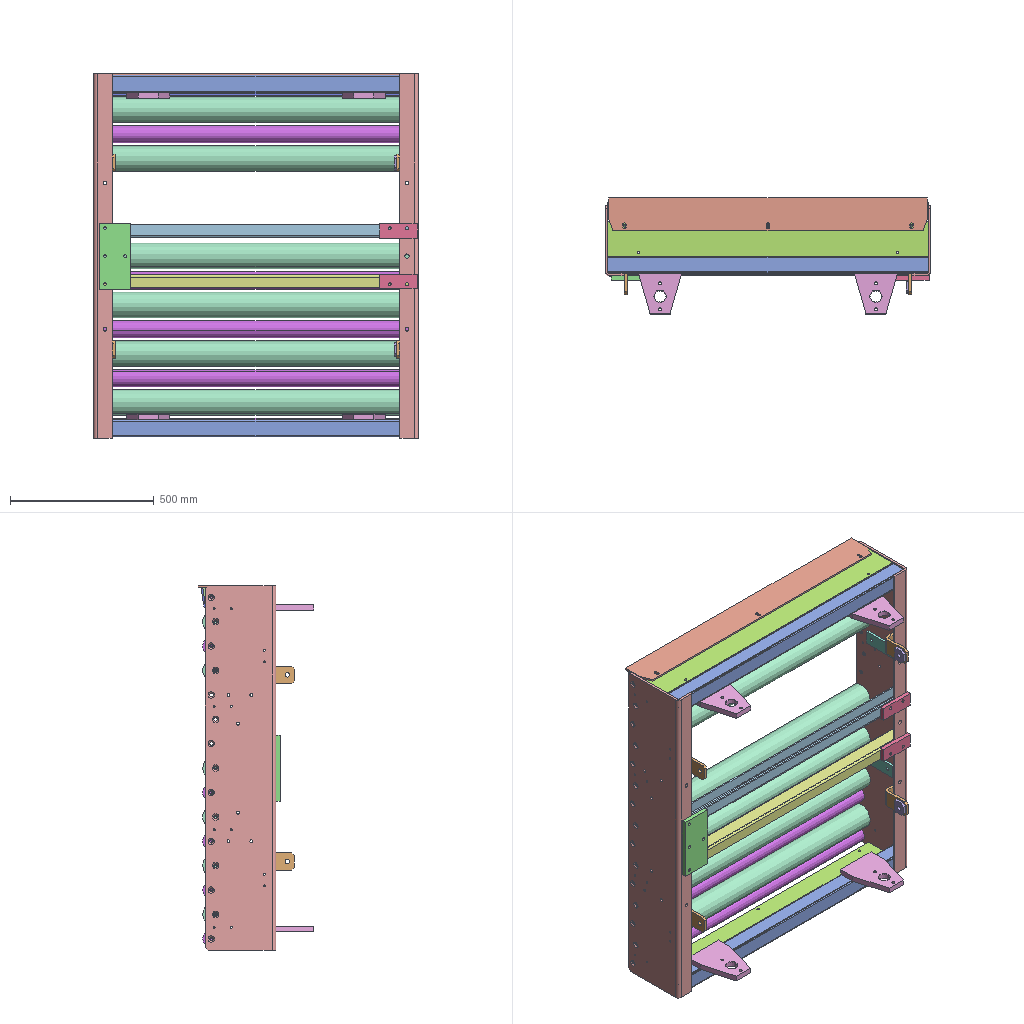Assembly | SolidWorks | 19 different items | 46 placed | box 1132 x 402 x 1271 mm
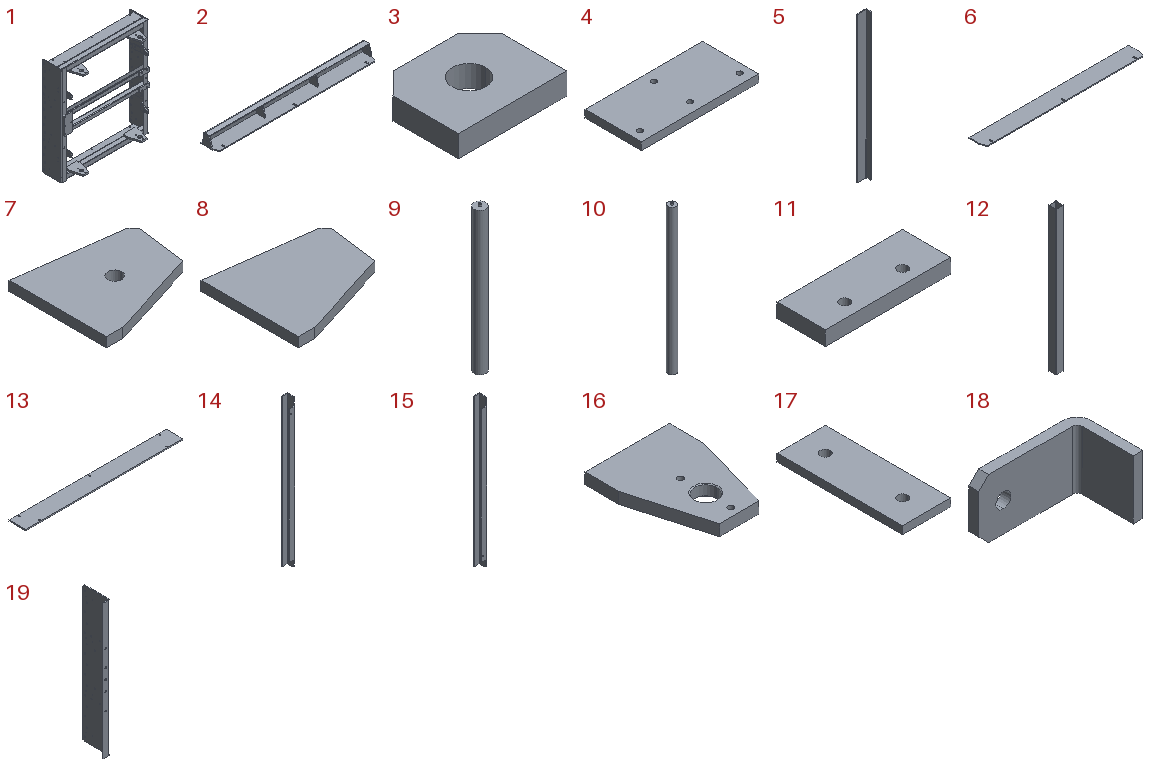Parts list (item | name | quantity | parent item | size | volume | features):
1 | (subassembly) | x1 | - | 1132 x 377 x 1270 mm | 14549074 mm3 | features CompositeCurve 3
2 | (subassembly) | x1 | - | 1116 x 115 x 79.93 mm | 1540136 mm3 | -
3 | - | x2 | in 1 | 50 x 40 x 10 mm | 17113 mm3 | features Chamfer 1, Extrusion 1, HoleWzd 1
4 | - | x1 | in 1 | 230 x 110 x 15 mm | 374597 mm3 | features Extrusion 1, HoleWzd 1
5 | - | x1 | in 2 | 75 x 40 x 1110 mm | 705931 mm3 | features Extrusion 1
6 | - | x1 | in 2 | 1110 x 115 x 6 mm | 758807 mm3 | features Extrusion 1, ICE 1
7 | - | x2 | in 2 | 67.858 x 60 x 6 mm | 18679 mm3 | features Chamfer 1, Extrusion 1, HoleWzd 1
8 | - | x2 | in 2 | 67.858 x 60 x 6 mm | 19020 mm3 | features Chamfer 1, Extrusion 1
9 | - | x7 | - | 89 x 89 x 1116 mm | 6784916 mm3 | features HoleWzd 2, ICE 2, Extrusion 1
10 | - | x6 | - | 60 x 60 x 1116 mm | 3085777 mm3 | features HoleWzd 2, ICE 2, Extrusion 1
11 | - | x2 | in 1 | 130 x 50 x 15 mm | 95049 mm3 | features Extrusion 1, HoleWzd 1
12 | - | x2 | in 1 | 60 x 60 x 1116 mm | 976944 mm3 | features Extrusion 1, Fillet 1, Shell 1
13 | - | x2 | in 1 | 1116 x 120 x 8 mm | 1069090 mm3 | features Extrusion 1, HoleWzd 1
14 | - | x1 | in 1 | 45 x 60 x 1116 mm | 728504 mm3 | features ICE 2, Extrusion 1, Fillet 1, HoleWzd 1
15 | - | x1 | in 1 | 45 x 60 x 1116 mm | 728477 mm3 | features ICE 2, Chamfer 1, Extrusion 1, HoleWzd 1
16 | - | x4 | in 1 | 150 x 200 x 20 mm | 459309 mm3 | features Chamfer 1, Extrusion 1, HoleWzd 1
17 | - | x4 | in 1 | 50 x 130 x 8 mm | 50693 mm3 | features Extrusion 1, HoleWzd 1
18 | - | x4 | in 1 | 110 x 67 x 60 mm | 94738 mm3 | features Chamfer 1, Extrusion 1, HoleWzd 1
19 | - | x2 | in 1 | 65 x 245 x 1270 mm | 2991073 mm3 | features ICE 4, HoleWzd 2, Chamfer 1, Extrusion 1
Mates (type | each side: item.copy, entity, surface, feature):
In the top assembly
Concentric | 19.1 face cylinder Cut-Extrude1 | 10.1 face cylinder Boss-Extrude1
Concentric | 19.1 face cylinder Cut-Extrude1 | 10.2 face cylinder Boss-Extrude1
Concentric | 19.1 edge | 10.3 face cylinder Boss-Extrude1
Concentric | 19.1 face cylinder Cut-Extrude1 | 10.4 face cylinder Boss-Extrude1
Concentric | 19.1 face cylinder Cut-Extrude1 | 9.1 face cylinder Boss-Extrude1
Concentric | 19.1 face cylinder Cut-Extrude1 | 9.2 face cylinder Boss-Extrude1
Concentric | 19.1 face cylinder Cut-Extrude1 | 9.3 face cylinder Boss-Extrude1
Concentric | 19.1 face cylinder Cut-Extrude1 | 9.4 face cylinder Boss-Extrude1
Concentric | 19.1 face cylinder Cut-Extrude1 | 9.5 face cylinder Boss-Extrude1
Concentric | 19.1 face cylinder Cut-Extrude1 | 9.6 face cylinder Boss-Extrude1
Concentric | 19.1 face cylinder Cut-Extrude1 | 9.7 face cylinder Boss-Extrude1
Concentric | 19.1 face cylinder Cut-Extrude1 | 10.5 face cylinder Boss-Extrude1
Concentric | 19.1 edge | 10.6 face cylinder Boss-Extrude1
Coincident | 10.1 face plane Boss-Extrude1 | 9.1 face plane Boss-Extrude1
Coincident | 10.1 face plane Boss-Extrude1 | 9.2 face plane Boss-Extrude1
Coincident | 9.2 face plane Boss-Extrude1 | 9.3 face plane Boss-Extrude1
Coincident | 10.2 face plane Boss-Extrude1 | 9.3 face plane Boss-Extrude1
Coincident | 10.2 face plane Boss-Extrude1 | 9.4 face plane Boss-Extrude1
Coincident | 10.3 face plane Boss-Extrude1 | 9.4 face plane Boss-Extrude1
Coincident | 10.3 face plane Boss-Extrude1 | 9.5 face plane Boss-Extrude1
Coincident | 10.5 face plane Boss-Extrude1 | 9.5 face plane Boss-Extrude1
Coincident | 10.5 face plane Boss-Extrude1 | 9.7 face plane Boss-Extrude1
Coincident | 10.4 face plane Boss-Extrude1 | 9.7 face plane Boss-Extrude1
Coincident | 10.4 face plane Boss-Extrude1 | 9.6 face plane Boss-Extrude1
Coincident | 10.6 face plane Boss-Extrude1 | 9.6 face plane Boss-Extrude1
Width | 9.1 face plane Boss-Extrude1 | 9.1 face plane Boss-Extrude1 | 19.1 face plane Boss-Extrude1 | 19.2 face plane Boss-Extrude1
Concentric | 19.1 face cylinder Cut-Extrude1 | 7.1 face cylinder M10 Tapped Hole2
Parallel | 13.1 face plane Boss-Extrude1 | 6.1 face plane Boss-Extrude1
Width | 7.1 face plane Boss-Extrude1 | 7.2 face plane Boss-Extrude1 | 19.2 face plane Boss-Extrude1 | 19.1 face plane Boss-Extrude1
In subassembly 1
Coincident | 19.3 face plane Boss-Extrude1 | 19.4 face plane Boss-Extrude1 | 2 times
Coincident | 19.4 face plane Boss-Extrude1 | 12.1 face plane Boss-Extrude1
Coincident | 19.3 face plane Boss-Extrude1 | 12.1 face plane Boss-Extrude1 | 2 times
Coincident | 19.4 face plane Boss-Extrude1 | 12.2 face plane Boss-Extrude1
Coincident | 12.1 face plane Boss-Extrude1 | 12.2 face plane Boss-Extrude1
DistanceDim | 12.2 face plane Boss-Extrude1 | 19.4 face plane Boss-Extrude1
DistanceDim | 12.1 face plane Boss-Extrude1 | 19.4 face plane Boss-Extrude1
Coincident | 19.4 face plane Boss-Extrude1 | 13.2 face plane Boss-Extrude1
Coincident | 12.1 face plane Boss-Extrude1 | 13.2 face plane Boss-Extrude1 | 2 times
Coincident | 12.2 face plane Boss-Extrude1 | 13.3 face plane Boss-Extrude1
Coincident | 19.4 face plane Boss-Extrude1 | 13.3 face plane Boss-Extrude1
Coincident | 13.2 face plane Boss-Extrude1 | 13.3 face plane Boss-Extrude1
Coincident | 12.2 face plane Boss-Extrude1 | 16.1 face plane Boss-Extrude1 | 2 times
Coincident | 16.1 face plane Boss-Extrude1 | 16.2 face plane Boss-Extrude1
Coincident | 16.1 face plane Boss-Extrude1 | 16.3 face plane Boss-Extrude1 | 2 times
Coincident | 16.1 face plane Boss-Extrude1 | 16.4 face plane Boss-Extrude1 | 2 times
Coincident | 12.1 face plane Boss-Extrude1 | 16.3 face plane Boss-Extrude1
Coincident | 12.1 face plane Boss-Extrude1 | 16.2 face plane Boss-Extrude1
Coincident | 16.2 face plane Boss-Extrude1 | 16.4 face plane Boss-Extrude1
DistanceDim | 16.4 face cylinder Boss-Extrude1 | 16.1 face cylinder Boss-Extrude1
Width | 16.4 face plane Boss-Extrude1 | 16.1 face plane Boss-Extrude1 | 19.4 face plane Boss-Extrude1 | 19.3 face plane Boss-Extrude1
Coincident | 19.3 face plane Boss-Extrude1 | 17.1 face plane Boss-Extrude1
Concentric | 19.3 face cylinder M12 Tapped Hole1 | 17.1 face cylinder M12 Tapped Hole1
Coincident | 19.3 face cylinder M12 Tapped Hole1 | 17.1 edge
Coincident | 17.1 face plane Boss-Extrude1 | 17.2 face plane Boss-Extrude1
Concentric | 19.3 face cylinder M12 Tapped Hole1 | 17.2 face cylinder M12 Tapped Hole1 | 2 times
Coincident | 19.4 face plane Boss-Extrude1 | 17.3 face plane Boss-Extrude1
Coincident | 19.4 face plane Boss-Extrude1 | 17.4 face plane Boss-Extrude1
Coincident | 19.4 face cylinder M12 Tapped Hole1 | 17.3 edge
Concentric | 19.4 face cylinder M12 Tapped Hole1 | 17.3 face cylinder M12 Tapped Hole1
Concentric | 19.4 face cylinder M12 Tapped Hole1 | 17.4 face cylinder M12 Tapped Hole1 | 2 times
Coincident | 19.4 face plane Boss-Extrude1 | 18.1 face plane Boss-Extrude1
DistanceDim | 18.1 face plane Boss-Extrude1 | 19.4 face plane Boss-Extrude1
Coincident | 18.1 face plane Boss-Extrude1 | 18.2 face plane Boss-Extrude1 | 2 times
Coincident | 18.3 face plane Boss-Extrude1 | 18.2 face plane Boss-Extrude1
Coincident | 18.2 face plane Boss-Extrude1 | 18.4 face plane Boss-Extrude1 | 2 times
Coincident | 18.1 face plane Boss-Extrude1 | 18.3 face plane Boss-Extrude1
Coincident | 19.3 face plane Boss-Extrude1 | 18.3 face plane Boss-Extrude1
Coincident | 18.3 face plane Boss-Extrude1 | 18.4 face plane Boss-Extrude1
DistanceDim | 18.1 face plane Boss-Extrude1 | 18.2 face plane Boss-Extrude1
Width | 18.1 face plane Boss-Extrude1 | 18.2 face plane Boss-Extrude1 | 13.2 face plane Boss-Extrude1 | 13.3 face plane Boss-Extrude1
Coincident | 3.1 face plane Boss-Extrude1 | 3.2 face plane Boss-Extrude1
Coincident | 18.4 face plane Boss-Extrude1 | 3.2 face plane Boss-Extrude1
Coincident | 19.4 face plane Boss-Extrude1 | 4.1 face plane Boss-Extrude1
Concentric | 19.4 face cylinder Cut-Extrude4 | 4.1 face cylinder M12 Tapped Hole2 | 2 times
Coincident | 19.3 face plane Boss-Extrude1 | 11.1 face plane Boss-Extrude1
Coincident | 11.1 face plane Boss-Extrude1 | 11.2 face plane Boss-Extrude1
Coincident | 19.4 face plane Boss-Extrude1 | 15.1 face plane Boss-Extrude1
Coincident | 19.3 face plane Boss-Extrude1 | 14.1 face plane Boss-Extrude1
Coincident | 14.1 face plane Boss-Extrude1 | 15.1 face plane Boss-Extrude1
Coincident | 11.2 face plane Boss-Extrude1 | 14.1 face plane Boss-Extrude1
DistanceDim | 14.1 face plane Boss-Extrude1 | 15.1 face plane Boss-Extrude1
Width | 14.1 face plane Boss-Extrude1 | 15.1 face plane Boss-Extrude1 | 13.3 face plane Boss-Extrude1 | 13.2 face plane Boss-Extrude1
Concentric | 19.3 face cylinder Cut-Extrude4 | 11.2 face cylinder M12 Tapped Hole1
Concentric | 19.3 face cylinder Cut-Extrude4 | 11.1 face cylinder M12 Tapped Hole1
Parallel | 19.3 face plane Boss-Extrude1 | 11.2 face plane Boss-Extrude1
Parallel | 19.3 face plane Boss-Extrude1 | 11.1 face plane Boss-Extrude1
In subassembly 2
Coincident | 6.2 face plane Boss-Extrude1 | 5.1 face plane Boss-Extrude1
Coincident | 6.2 face plane Boss-Extrude1 | 5.1 edge
DistanceDim | 5.1 edge | 6.2 face plane Boss-Extrude1
DistanceDim | 7.3 face plane Boss-Extrude1 | 6.2 face plane Boss-Extrude1
Coincident | 6.2 face plane Boss-Extrude1 | 7.4 face plane Boss-Extrude1
Coincident | 5.1 edge | 7.4 edge
DistanceDim | 7.4 face plane Boss-Extrude1 | 5.1 face plane Boss-Extrude1
Coincident | 6.2 face plane Boss-Extrude1 | 8.1 face plane Boss-Extrude1
Coincident | 7.3 face plane Boss-Extrude1 | 8.1 face plane Boss-Extrude1
Coincident | 6.2 face plane Boss-Extrude1 | 8.2 face plane Boss-Extrude1
Coincident | 8.1 face plane Boss-Extrude1 | 8.2 face plane Boss-Extrude1
DistanceDim | 7.3 face plane Boss-Extrude1 | 8.1 face plane Boss-Extrude1
DistanceDim | 8.2 face plane Boss-Extrude1 | 7.4 face plane Boss-Extrude1
Coincident | 7.4 face plane Boss-Extrude1 | 7.3 face plane Boss-Extrude1 | 2 times